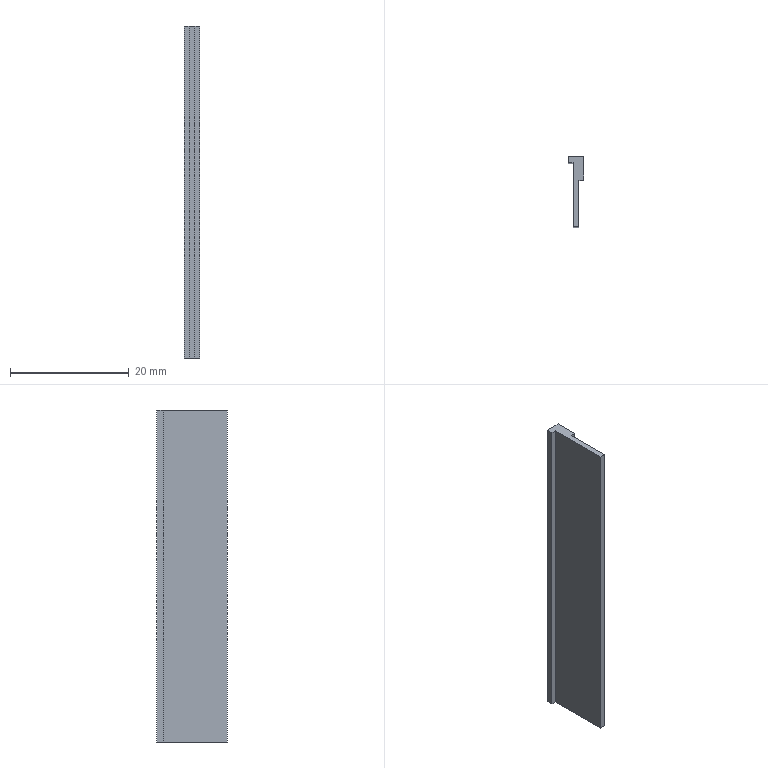Part | NX | features BREP 2 | 2 solids | 20 faces | box 2.58 x 11.896 x 56 mm | volume 1761 mm3 | plane 20
STEP:
#1=CARTESIAN_POINT('',(-0.4899,4.83,-4.));
#2=VERTEX_POINT('',#1);
#3=CARTESIAN_POINT('',(-0.4899,4.83,52.));
#4=VERTEX_POINT('',#3);
#5=CARTESIAN_POINT('',(-0.4899,4.83,0.));
#6=DIRECTION('',(0.,0.,1.));
#7=VECTOR('',#6,1000.);
#8=LINE('',#5,#7);
#9=EDGE_CURVE('',#2,#4,#8,.T.);
#10=ORIENTED_EDGE('',*,*,#9,.T.);
#11=CARTESIAN_POINT('',(-1.29,4.83,52.));
#12=VERTEX_POINT('',#11);
#13=CARTESIAN_POINT('',(-7.04,4.83,52.));
#14=DIRECTION('',(1.,0.,0.));
#15=VECTOR('',#14,1000.);
#16=LINE('',#13,#15);
#17=EDGE_CURVE('',#12,#4,#16,.T.);
#18=ORIENTED_EDGE('',*,*,#17,.F.);
#19=CARTESIAN_POINT('',(-1.29,4.83,-4.));
#20=VERTEX_POINT('',#19);
#21=CARTESIAN_POINT('',(-1.29,4.83,0.));
#22=DIRECTION('',(0.,0.,1.));
#23=VECTOR('',#22,1000.);
#24=LINE('',#21,#23);
#25=EDGE_CURVE('',#20,#12,#24,.T.);
#26=ORIENTED_EDGE('',*,*,#25,.F.);
#27=CARTESIAN_POINT('',(-7.04,4.83,-4.));
#28=DIRECTION('',(1.,0.,0.));
#29=VECTOR('',#28,1000.);
#30=LINE('',#27,#29);
#31=EDGE_CURVE('',#20,#2,#30,.T.);
#32=ORIENTED_EDGE('',*,*,#31,.T.);
#33=EDGE_LOOP('',(#10,#18,#26,#32));
#34=FACE_BOUND('',#33,.T.);
#35=CARTESIAN_POINT('',(-0.4899,4.83,0.));
#36=DIRECTION('',(0.,1.,0.));
#37=DIRECTION('',(1.,0.,0.));
#38=AXIS2_PLACEMENT_3D('',#35,#36,#37);
#39=PLANE('',#38);
#40=ADVANCED_FACE('',(#34),#39,.F.);
#41=ORIENTED_EDGE('',*,*,#25,.T.);
#42=CARTESIAN_POINT('',(-1.29,5.923,52.));
#43=VERTEX_POINT('',#42);
#44=CARTESIAN_POINT('',(-1.29,-19.679,52.));
#45=DIRECTION('',(0.,-1.,0.));
#46=VECTOR('',#45,1000.);
#47=LINE('',#44,#46);
#48=EDGE_CURVE('',#43,#12,#47,.T.);
#49=ORIENTED_EDGE('',*,*,#48,.F.);
#50=CARTESIAN_POINT('',(-1.29,5.923,-4.));
#51=VERTEX_POINT('',#50);
#52=CARTESIAN_POINT('',(-1.29,5.923,0.));
#53=DIRECTION('',(0.,0.,1.));
#54=VECTOR('',#53,1000.);
#55=LINE('',#52,#54);
#56=EDGE_CURVE('',#51,#43,#55,.T.);
#57=ORIENTED_EDGE('',*,*,#56,.F.);
#58=CARTESIAN_POINT('',(-1.29,-19.679,-4.));
#59=DIRECTION('',(0.,-1.,0.));
#60=VECTOR('',#59,1000.);
#61=LINE('',#58,#60);
#62=EDGE_CURVE('',#51,#20,#61,.T.);
#63=ORIENTED_EDGE('',*,*,#62,.T.);
#64=EDGE_LOOP('',(#41,#49,#57,#63));
#65=FACE_BOUND('',#64,.T.);
#66=CARTESIAN_POINT('',(-1.29,4.83,0.));
#67=DIRECTION('',(1.,0.,0.));
#68=DIRECTION('',(0.,-1.,0.));
#69=AXIS2_PLACEMENT_3D('',#66,#67,#68);
#70=PLANE('',#69);
#71=ADVANCED_FACE('',(#65),#70,.F.);
#72=ORIENTED_EDGE('',*,*,#56,.T.);
#73=CARTESIAN_POINT('',(1.29,5.923,52.));
#74=VERTEX_POINT('',#73);
#75=CARTESIAN_POINT('',(-7.04,5.923,52.));
#76=DIRECTION('',(-1.,0.,0.));
#77=VECTOR('',#76,1000.);
#78=LINE('',#75,#77);
#79=EDGE_CURVE('',#74,#43,#78,.T.);
#80=ORIENTED_EDGE('',*,*,#79,.F.);
#81=CARTESIAN_POINT('',(1.29,5.923,-4.));
#82=VERTEX_POINT('',#81);
#83=CARTESIAN_POINT('',(1.29,5.923,0.));
#84=DIRECTION('',(0.,0.,1.));
#85=VECTOR('',#84,1000.);
#86=LINE('',#83,#85);
#87=EDGE_CURVE('',#82,#74,#86,.T.);
#88=ORIENTED_EDGE('',*,*,#87,.F.);
#89=CARTESIAN_POINT('',(-7.04,5.923,-4.));
#90=DIRECTION('',(-1.,0.,0.));
#91=VECTOR('',#90,1000.);
#92=LINE('',#89,#91);
#93=EDGE_CURVE('',#82,#51,#92,.T.);
#94=ORIENTED_EDGE('',*,*,#93,.T.);
#95=EDGE_LOOP('',(#72,#80,#88,#94));
#96=FACE_BOUND('',#95,.T.);
#97=CARTESIAN_POINT('',(-7.04,5.923,0.));
#98=DIRECTION('',(0.,1.,0.));
#99=DIRECTION('',(1.,0.,0.));
#100=AXIS2_PLACEMENT_3D('',#97,#98,#99);
#101=PLANE('',#100);
#102=ADVANCED_FACE('',(#96),#101,.T.);
#103=ORIENTED_EDGE('',*,*,#87,.T.);
#104=CARTESIAN_POINT('',(1.29,1.93,52.));
#105=VERTEX_POINT('',#104);
#106=CARTESIAN_POINT('',(1.29,-19.679,52.));
#107=DIRECTION('',(0.,1.,0.));
#108=VECTOR('',#107,1000.);
#109=LINE('',#106,#108);
#110=EDGE_CURVE('',#105,#74,#109,.T.);
#111=ORIENTED_EDGE('',*,*,#110,.F.);
#112=CARTESIAN_POINT('',(1.29,1.93,-4.));
#113=VERTEX_POINT('',#112);
#114=CARTESIAN_POINT('',(1.29,1.93,0.));
#115=DIRECTION('',(0.,0.,1.));
#116=VECTOR('',#115,1000.);
#117=LINE('',#114,#116);
#118=EDGE_CURVE('',#113,#105,#117,.T.);
#119=ORIENTED_EDGE('',*,*,#118,.F.);
#120=CARTESIAN_POINT('',(1.29,-19.679,-4.));
#121=DIRECTION('',(0.,1.,0.));
#122=VECTOR('',#121,1000.);
#123=LINE('',#120,#122);
#124=EDGE_CURVE('',#113,#82,#123,.T.);
#125=ORIENTED_EDGE('',*,*,#124,.T.);
#126=EDGE_LOOP('',(#103,#111,#119,#125));
#127=FACE_BOUND('',#126,.T.);
#128=CARTESIAN_POINT('',(1.29,5.923,0.));
#129=DIRECTION('',(-1.,0.,0.));
#130=DIRECTION('',(0.,1.,0.));
#131=AXIS2_PLACEMENT_3D('',#128,#129,#130);
#132=PLANE('',#131);
#133=ADVANCED_FACE('',(#127),#132,.F.);
#134=ORIENTED_EDGE('',*,*,#118,.T.);
#135=CARTESIAN_POINT('',(0.4899,1.93,52.));
#136=VERTEX_POINT('',#135);
#137=CARTESIAN_POINT('',(-7.04,1.93,52.));
#138=DIRECTION('',(1.,0.,0.));
#139=VECTOR('',#138,1000.);
#140=LINE('',#137,#139);
#141=EDGE_CURVE('',#136,#105,#140,.T.);
#142=ORIENTED_EDGE('',*,*,#141,.F.);
#143=CARTESIAN_POINT('',(0.4899,1.93,-4.));
#144=VERTEX_POINT('',#143);
#145=CARTESIAN_POINT('',(0.4899,1.93,0.));
#146=DIRECTION('',(0.,0.,1.));
#147=VECTOR('',#146,1000.);
#148=LINE('',#145,#147);
#149=EDGE_CURVE('',#144,#136,#148,.T.);
#150=ORIENTED_EDGE('',*,*,#149,.F.);
#151=CARTESIAN_POINT('',(-7.04,1.93,-4.));
#152=DIRECTION('',(1.,0.,0.));
#153=VECTOR('',#152,1000.);
#154=LINE('',#151,#153);
#155=EDGE_CURVE('',#144,#113,#154,.T.);
#156=ORIENTED_EDGE('',*,*,#155,.T.);
#157=EDGE_LOOP('',(#134,#142,#150,#156));
#158=FACE_BOUND('',#157,.T.);
#159=CARTESIAN_POINT('',(1.29,1.93,0.));
#160=DIRECTION('',(0.,1.,0.));
#161=DIRECTION('',(1.,0.,0.));
#162=AXIS2_PLACEMENT_3D('',#159,#160,#161);
#163=PLANE('',#162);
#164=ADVANCED_FACE('',(#158),#163,.F.);
#165=CARTESIAN_POINT('',(0.4899,-5.973,-4.));
#166=VERTEX_POINT('',#165);
#167=CARTESIAN_POINT('',(0.4899,-5.973,52.));
#168=VERTEX_POINT('',#167);
#169=CARTESIAN_POINT('',(0.4899,-5.973,0.));
#170=DIRECTION('',(0.,0.,1.));
#171=VECTOR('',#170,1000.);
#172=LINE('',#169,#171);
#173=EDGE_CURVE('',#166,#168,#172,.T.);
#174=ORIENTED_EDGE('',*,*,#173,.F.);
#175=CARTESIAN_POINT('',(0.4899,-19.679,-4.));
#176=DIRECTION('',(0.,1.,0.));
#177=VECTOR('',#176,1000.);
#178=LINE('',#175,#177);
#179=EDGE_CURVE('',#166,#144,#178,.T.);
#180=ORIENTED_EDGE('',*,*,#179,.T.);
#181=ORIENTED_EDGE('',*,*,#149,.T.);
#182=CARTESIAN_POINT('',(0.4899,-19.679,52.));
#183=DIRECTION('',(0.,1.,0.));
#184=VECTOR('',#183,1000.);
#185=LINE('',#182,#184);
#186=EDGE_CURVE('',#168,#136,#185,.T.);
#187=ORIENTED_EDGE('',*,*,#186,.F.);
#188=EDGE_LOOP('',(#174,#180,#181,#187));
#189=FACE_BOUND('',#188,.T.);
#190=CARTESIAN_POINT('',(0.4899,-5.28,0.));
#191=DIRECTION('',(-1.,0.,0.));
#192=DIRECTION('',(0.,1.,0.));
#193=AXIS2_PLACEMENT_3D('',#190,#191,#192);
#194=PLANE('',#193);
#195=ADVANCED_FACE('',(#189),#194,.F.);
#196=ORIENTED_EDGE('',*,*,#173,.T.);
#197=CARTESIAN_POINT('',(-0.4899,-5.973,52.));
#198=VERTEX_POINT('',#197);
#199=CARTESIAN_POINT('',(-7.04,-5.973,52.));
#200=DIRECTION('',(1.,0.,0.));
#201=VECTOR('',#200,1000.);
#202=LINE('',#199,#201);
#203=EDGE_CURVE('',#198,#168,#202,.T.);
#204=ORIENTED_EDGE('',*,*,#203,.F.);
#205=CARTESIAN_POINT('',(-0.4899,-5.973,-4.));
#206=VERTEX_POINT('',#205);
#207=CARTESIAN_POINT('',(-0.4899,-5.973,0.));
#208=DIRECTION('',(0.,0.,1.));
#209=VECTOR('',#208,1000.);
#210=LINE('',#207,#209);
#211=EDGE_CURVE('',#206,#198,#210,.T.);
#212=ORIENTED_EDGE('',*,*,#211,.F.);
#213=CARTESIAN_POINT('',(-7.04,-5.973,-4.));
#214=DIRECTION('',(1.,0.,0.));
#215=VECTOR('',#214,1000.);
#216=LINE('',#213,#215);
#217=EDGE_CURVE('',#206,#166,#216,.T.);
#218=ORIENTED_EDGE('',*,*,#217,.T.);
#219=EDGE_LOOP('',(#196,#204,#212,#218));
#220=FACE_BOUND('',#219,.T.);
#221=CARTESIAN_POINT('',(-7.04,-5.973,0.));
#222=DIRECTION('',(0.,-1.,0.));
#223=DIRECTION('',(-1.,0.,0.));
#224=AXIS2_PLACEMENT_3D('',#221,#222,#223);
#225=PLANE('',#224);
#226=ADVANCED_FACE('',(#220),#225,.T.);
#227=CARTESIAN_POINT('',(-0.4899,-19.679,-4.));
#228=DIRECTION('',(0.,-1.,0.));
#229=VECTOR('',#228,1000.);
#230=LINE('',#227,#229);
#231=EDGE_CURVE('',#2,#206,#230,.T.);
#232=ORIENTED_EDGE('',*,*,#231,.T.);
#233=ORIENTED_EDGE('',*,*,#211,.T.);
#234=CARTESIAN_POINT('',(-0.4899,-19.679,52.));
#235=DIRECTION('',(0.,-1.,0.));
#236=VECTOR('',#235,1000.);
#237=LINE('',#234,#236);
#238=EDGE_CURVE('',#4,#198,#237,.T.);
#239=ORIENTED_EDGE('',*,*,#238,.F.);
#240=ORIENTED_EDGE('',*,*,#9,.F.);
#241=EDGE_LOOP('',(#232,#233,#239,#240));
#242=FACE_BOUND('',#241,.T.);
#243=CARTESIAN_POINT('',(-0.4899,-2.38,0.));
#244=DIRECTION('',(1.,0.,0.));
#245=DIRECTION('',(0.,-1.,0.));
#246=AXIS2_PLACEMENT_3D('',#243,#244,#245);
#247=PLANE('',#246);
#248=ADVANCED_FACE('',(#242),#247,.F.);
#249=ORIENTED_EDGE('',*,*,#238,.T.);
#250=ORIENTED_EDGE('',*,*,#203,.T.);
#251=ORIENTED_EDGE('',*,*,#186,.T.);
#252=ORIENTED_EDGE('',*,*,#141,.T.);
#253=ORIENTED_EDGE('',*,*,#110,.T.);
#254=ORIENTED_EDGE('',*,*,#79,.T.);
#255=ORIENTED_EDGE('',*,*,#48,.T.);
#256=ORIENTED_EDGE('',*,*,#17,.T.);
#257=EDGE_LOOP('',(#249,#250,#251,#252,#253,#254,#255,#256));
#258=FACE_BOUND('',#257,.T.);
#259=CARTESIAN_POINT('',(-7.04,-19.679,52.));
#260=DIRECTION('',(0.,0.,1.));
#261=DIRECTION('',(-1.,0.,0.));
#262=AXIS2_PLACEMENT_3D('',#259,#260,#261);
#263=PLANE('',#262);
#264=ADVANCED_FACE('',(#258),#263,.T.);
#265=ORIENTED_EDGE('',*,*,#217,.F.);
#266=ORIENTED_EDGE('',*,*,#231,.F.);
#267=ORIENTED_EDGE('',*,*,#31,.F.);
#268=ORIENTED_EDGE('',*,*,#62,.F.);
#269=ORIENTED_EDGE('',*,*,#93,.F.);
#270=ORIENTED_EDGE('',*,*,#124,.F.);
#271=ORIENTED_EDGE('',*,*,#155,.F.);
#272=ORIENTED_EDGE('',*,*,#179,.F.);
#273=EDGE_LOOP('',(#265,#266,#267,#268,#269,#270,#271,#272));
#274=FACE_BOUND('',#273,.T.);
#275=CARTESIAN_POINT('',(-7.04,-19.679,-4.));
#276=DIRECTION('',(0.,0.,1.));
#277=DIRECTION('',(-1.,0.,0.));
#278=AXIS2_PLACEMENT_3D('',#275,#276,#277);
#279=PLANE('',#278);
#280=ADVANCED_FACE('',(#274),#279,.F.);
#281=CLOSED_SHELL('',(#40,#71,#102,#133,#164,#195,#226,#248,#264,#280));
#282=MANIFOLD_SOLID_BREP('',#281);
#283=CARTESIAN_POINT('',(-0.4899,4.83,-4.));
#284=VERTEX_POINT('',#283);
#285=CARTESIAN_POINT('',(-0.4899,4.83,52.));
#286=VERTEX_POINT('',#285);
#287=CARTESIAN_POINT('',(-0.4899,4.83,0.));
#288=DIRECTION('',(0.,0.,1.));
#289=VECTOR('',#288,1000.);
#290=LINE('',#287,#289);
#291=EDGE_CURVE('',#284,#286,#290,.T.);
#292=ORIENTED_EDGE('',*,*,#291,.T.);
#293=CARTESIAN_POINT('',(-1.29,4.83,52.));
#294=VERTEX_POINT('',#293);
#295=CARTESIAN_POINT('',(-7.04,4.83,52.));
#296=DIRECTION('',(1.,0.,0.));
#297=VECTOR('',#296,1000.);
#298=LINE('',#295,#297);
#299=EDGE_CURVE('',#294,#286,#298,.T.);
#300=ORIENTED_EDGE('',*,*,#299,.F.);
#301=CARTESIAN_POINT('',(-1.29,4.83,-4.));
#302=VERTEX_POINT('',#301);
#303=CARTESIAN_POINT('',(-1.29,4.83,0.));
#304=DIRECTION('',(0.,0.,1.));
#305=VECTOR('',#304,1000.);
#306=LINE('',#303,#305);
#307=EDGE_CURVE('',#302,#294,#306,.T.);
#308=ORIENTED_EDGE('',*,*,#307,.F.);
#309=CARTESIAN_POINT('',(-7.04,4.83,-4.));
#310=DIRECTION('',(1.,0.,0.));
#311=VECTOR('',#310,1000.);
#312=LINE('',#309,#311);
#313=EDGE_CURVE('',#302,#284,#312,.T.);
#314=ORIENTED_EDGE('',*,*,#313,.T.);
#315=EDGE_LOOP('',(#292,#300,#308,#314));
#316=FACE_BOUND('',#315,.T.);
#317=CARTESIAN_POINT('',(-0.4899,4.83,0.));
#318=DIRECTION('',(0.,1.,0.));
#319=DIRECTION('',(1.,0.,0.));
#320=AXIS2_PLACEMENT_3D('',#317,#318,#319);
#321=PLANE('',#320);
#322=ADVANCED_FACE('',(#316),#321,.F.);
#323=ORIENTED_EDGE('',*,*,#307,.T.);
#324=CARTESIAN_POINT('',(-1.29,5.923,52.));
#325=VERTEX_POINT('',#324);
#326=CARTESIAN_POINT('',(-1.29,-19.679,52.));
#327=DIRECTION('',(0.,-1.,0.));
#328=VECTOR('',#327,1000.);
#329=LINE('',#326,#328);
#330=EDGE_CURVE('',#325,#294,#329,.T.);
#331=ORIENTED_EDGE('',*,*,#330,.F.);
#332=CARTESIAN_POINT('',(-1.29,5.923,-4.));
#333=VERTEX_POINT('',#332);
#334=CARTESIAN_POINT('',(-1.29,5.923,0.));
#335=DIRECTION('',(0.,0.,1.));
#336=VECTOR('',#335,1000.);
#337=LINE('',#334,#336);
#338=EDGE_CURVE('',#333,#325,#337,.T.);
#339=ORIENTED_EDGE('',*,*,#338,.F.);
#340=CARTESIAN_POINT('',(-1.29,-19.679,-4.));
#341=DIRECTION('',(0.,-1.,0.));
#342=VECTOR('',#341,1000.);
#343=LINE('',#340,#342);
#344=EDGE_CURVE('',#333,#302,#343,.T.);
#345=ORIENTED_EDGE('',*,*,#344,.T.);
#346=EDGE_LOOP('',(#323,#331,#339,#345));
#347=FACE_BOUND('',#346,.T.);
#348=CARTESIAN_POINT('',(-1.29,4.83,0.));
#349=DIRECTION('',(1.,0.,0.));
#350=DIRECTION('',(0.,-1.,0.));
#351=AXIS2_PLACEMENT_3D('',#348,#349,#350);
#352=PLANE('',#351);
#353=ADVANCED_FACE('',(#347),#352,.F.);
#354=ORIENTED_EDGE('',*,*,#338,.T.);
#355=CARTESIAN_POINT('',(1.29,5.923,52.));
#356=VERTEX_POINT('',#355);
#357=CARTESIAN_POINT('',(-7.04,5.923,52.));
#358=DIRECTION('',(-1.,0.,0.));
#359=VECTOR('',#358,1000.);
#360=LINE('',#357,#359);
#361=EDGE_CURVE('',#356,#325,#360,.T.);
#362=ORIENTED_EDGE('',*,*,#361,.F.);
#363=CARTESIAN_POINT('',(1.29,5.923,-4.));
#364=VERTEX_POINT('',#363);
#365=CARTESIAN_POINT('',(1.29,5.923,0.));
#366=DIRECTION('',(0.,0.,1.));
#367=VECTOR('',#366,1000.);
#368=LINE('',#365,#367);
#369=EDGE_CURVE('',#364,#356,#368,.T.);
#370=ORIENTED_EDGE('',*,*,#369,.F.);
#371=CARTESIAN_POINT('',(-7.04,5.923,-4.));
#372=DIRECTION('',(-1.,0.,0.));
#373=VECTOR('',#372,1000.);
#374=LINE('',#371,#373);
#375=EDGE_CURVE('',#364,#333,#374,.T.);
#376=ORIENTED_EDGE('',*,*,#375,.T.);
#377=EDGE_LOOP('',(#354,#362,#370,#376));
#378=FACE_BOUND('',#377,.T.);
#379=CARTESIAN_POINT('',(-7.04,5.923,0.));
#380=DIRECTION('',(0.,1.,0.));
#381=DIRECTION('',(1.,0.,0.));
#382=AXIS2_PLACEMENT_3D('',#379,#380,#381);
#383=PLANE('',#382);
#384=ADVANCED_FACE('',(#378),#383,.T.);
#385=ORIENTED_EDGE('',*,*,#369,.T.);
#386=CARTESIAN_POINT('',(1.29,1.93,52.));
#387=VERTEX_POINT('',#386);
#388=CARTESIAN_POINT('',(1.29,-19.679,52.));
#389=DIRECTION('',(0.,1.,0.));
#390=VECTOR('',#389,1000.);
#391=LINE('',#388,#390);
#392=EDGE_CURVE('',#387,#356,#391,.T.);
#393=ORIENTED_EDGE('',*,*,#392,.F.);
#394=CARTESIAN_POINT('',(1.29,1.93,-4.));
#395=VERTEX_POINT('',#394);
#396=CARTESIAN_POINT('',(1.29,1.93,0.));
#397=DIRECTION('',(0.,0.,1.));
#398=VECTOR('',#397,1000.);
#399=LINE('',#396,#398);
#400=EDGE_CURVE('',#395,#387,#399,.T.);
#401=ORIENTED_EDGE('',*,*,#400,.F.);
#402=CARTESIAN_POINT('',(1.29,-19.679,-4.));
#403=DIRECTION('',(0.,1.,0.));
#404=VECTOR('',#403,1000.);
#405=LINE('',#402,#404);
#406=EDGE_CURVE('',#395,#364,#405,.T.);
#407=ORIENTED_EDGE('',*,*,#406,.T.);
#408=EDGE_LOOP('',(#385,#393,#401,#407));
#409=FACE_BOUND('',#408,.T.);
#410=CARTESIAN_POINT('',(1.29,5.923,0.));
#411=DIRECTION('',(-1.,0.,0.));
#412=DIRECTION('',(0.,1.,0.));
#413=AXIS2_PLACEMENT_3D('',#410,#411,#412);
#414=PLANE('',#413);
#415=ADVANCED_FACE('',(#409),#414,.F.);
#416=ORIENTED_EDGE('',*,*,#400,.T.);
#417=CARTESIAN_POINT('',(0.4899,1.93,52.));
#418=VERTEX_POINT('',#417);
#419=CARTESIAN_POINT('',(-7.04,1.93,52.));
#420=DIRECTION('',(1.,0.,0.));
#421=VECTOR('',#420,1000.);
#422=LINE('',#419,#421);
#423=EDGE_CURVE('',#418,#387,#422,.T.);
#424=ORIENTED_EDGE('',*,*,#423,.F.);
#425=CARTESIAN_POINT('',(0.4899,1.93,-4.));
#426=VERTEX_POINT('',#425);
#427=CARTESIAN_POINT('',(0.4899,1.93,0.));
#428=DIRECTION('',(0.,0.,1.));
#429=VECTOR('',#428,1000.);
#430=LINE('',#427,#429);
#431=EDGE_CURVE('',#426,#418,#430,.T.);
#432=ORIENTED_EDGE('',*,*,#431,.F.);
#433=CARTESIAN_POINT('',(-7.04,1.93,-4.));
#434=DIRECTION('',(1.,0.,0.));
#435=VECTOR('',#434,1000.);
#436=LINE('',#433,#435);
#437=EDGE_CURVE('',#426,#395,#436,.T.);
#438=ORIENTED_EDGE('',*,*,#437,.T.);
#439=EDGE_LOOP('',(#416,#424,#432,#438));
#440=FACE_BOUND('',#439,.T.);
#441=CARTESIAN_POINT('',(1.29,1.93,0.));
#442=DIRECTION('',(0.,1.,0.));
#443=DIRECTION('',(1.,0.,0.));
#444=AXIS2_PLACEMENT_3D('',#441,#442,#443);
#445=PLANE('',#444);
#446=ADVANCED_FACE('',(#440),#445,.F.);
#447=CARTESIAN_POINT('',(0.4899,-5.973,-4.));
#448=VERTEX_POINT('',#447);
#449=CARTESIAN_POINT('',(0.4899,-5.973,52.));
#450=VERTEX_POINT('',#449);
#451=CARTESIAN_POINT('',(0.4899,-5.973,0.));
#452=DIRECTION('',(0.,0.,1.));
#453=VECTOR('',#452,1000.);
#454=LINE('',#451,#453);
#455=EDGE_CURVE('',#448,#450,#454,.T.);
#456=ORIENTED_EDGE('',*,*,#455,.F.);
#457=CARTESIAN_POINT('',(0.4899,-19.679,-4.));
#458=DIRECTION('',(0.,1.,0.));
#459=VECTOR('',#458,1000.);
#460=LINE('',#457,#459);
#461=EDGE_CURVE('',#448,#426,#460,.T.);
#462=ORIENTED_EDGE('',*,*,#461,.T.);
#463=ORIENTED_EDGE('',*,*,#431,.T.);
#464=CARTESIAN_POINT('',(0.4899,-19.679,52.));
#465=DIRECTION('',(0.,1.,0.));
#466=VECTOR('',#465,1000.);
#467=LINE('',#464,#466);
#468=EDGE_CURVE('',#450,#418,#467,.T.);
#469=ORIENTED_EDGE('',*,*,#468,.F.);
#470=EDGE_LOOP('',(#456,#462,#463,#469));
#471=FACE_BOUND('',#470,.T.);
#472=CARTESIAN_POINT('',(0.4899,-5.28,0.));
#473=DIRECTION('',(-1.,0.,0.));
#474=DIRECTION('',(0.,1.,0.));
#475=AXIS2_PLACEMENT_3D('',#472,#473,#474);
#476=PLANE('',#475);
#477=ADVANCED_FACE('',(#471),#476,.F.);
#478=ORIENTED_EDGE('',*,*,#455,.T.);
#479=CARTESIAN_POINT('',(-0.4899,-5.973,52.));
#480=VERTEX_POINT('',#479);
#481=CARTESIAN_POINT('',(-7.04,-5.973,52.));
#482=DIRECTION('',(1.,0.,0.));
#483=VECTOR('',#482,1000.);
#484=LINE('',#481,#483);
#485=EDGE_CURVE('',#480,#450,#484,.T.);
#486=ORIENTED_EDGE('',*,*,#485,.F.);
#487=CARTESIAN_POINT('',(-0.4899,-5.973,-4.));
#488=VERTEX_POINT('',#487);
#489=CARTESIAN_POINT('',(-0.4899,-5.973,0.));
#490=DIRECTION('',(0.,0.,1.));
#491=VECTOR('',#490,1000.);
#492=LINE('',#489,#491);
#493=EDGE_CURVE('',#488,#480,#492,.T.);
#494=ORIENTED_EDGE('',*,*,#493,.F.);
#495=CARTESIAN_POINT('',(-7.04,-5.973,-4.));
#496=DIRECTION('',(1.,0.,0.));
#497=VECTOR('',#496,1000.);
#498=LINE('',#495,#497);
#499=EDGE_CURVE('',#488,#448,#498,.T.);
#500=ORIENTED_EDGE('',*,*,#499,.T.);
#501=EDGE_LOOP('',(#478,#486,#494,#500));
#502=FACE_BOUND('',#501,.T.);
#503=CARTESIAN_POINT('',(-7.04,-5.973,0.));
#504=DIRECTION('',(0.,-1.,0.));
#505=DIRECTION('',(-1.,0.,0.));
#506=AXIS2_PLACEMENT_3D('',#503,#504,#505);
#507=PLANE('',#506);
#508=ADVANCED_FACE('',(#502),#507,.T.);
#509=CARTESIAN_POINT('',(-0.4899,-19.679,-4.));
#510=DIRECTION('',(0.,-1.,0.));
#511=VECTOR('',#510,1000.);
#512=LINE('',#509,#511);
#513=EDGE_CURVE('',#284,#488,#512,.T.);
#514=ORIENTED_EDGE('',*,*,#513,.T.);
#515=ORIENTED_EDGE('',*,*,#493,.T.);
#516=CARTESIAN_POINT('',(-0.4899,-19.679,52.));
#517=DIRECTION('',(0.,-1.,0.));
#518=VECTOR('',#517,1000.);
#519=LINE('',#516,#518);
#520=EDGE_CURVE('',#286,#480,#519,.T.);
#521=ORIENTED_EDGE('',*,*,#520,.F.);
#522=ORIENTED_EDGE('',*,*,#291,.F.);
#523=EDGE_LOOP('',(#514,#515,#521,#522));
#524=FACE_BOUND('',#523,.T.);
#525=CARTESIAN_POINT('',(-0.4899,-2.38,0.));
#526=DIRECTION('',(1.,0.,0.));
#527=DIRECTION('',(0.,-1.,0.));
#528=AXIS2_PLACEMENT_3D('',#525,#526,#527);
#529=PLANE('',#528);
#530=ADVANCED_FACE('',(#524),#529,.F.);
#531=ORIENTED_EDGE('',*,*,#520,.T.);
#532=ORIENTED_EDGE('',*,*,#485,.T.);
#533=ORIENTED_EDGE('',*,*,#468,.T.);
#534=ORIENTED_EDGE('',*,*,#423,.T.);
#535=ORIENTED_EDGE('',*,*,#392,.T.);
#536=ORIENTED_EDGE('',*,*,#361,.T.);
#537=ORIENTED_EDGE('',*,*,#330,.T.);
#538=ORIENTED_EDGE('',*,*,#299,.T.);
#539=EDGE_LOOP('',(#531,#532,#533,#534,#535,#536,#537,#538));
#540=FACE_BOUND('',#539,.T.);
#541=CARTESIAN_POINT('',(-7.04,-19.679,52.));
#542=DIRECTION('',(0.,0.,1.));
#543=DIRECTION('',(-1.,0.,0.));
#544=AXIS2_PLACEMENT_3D('',#541,#542,#543);
#545=PLANE('',#544);
#546=ADVANCED_FACE('',(#540),#545,.T.);
#547=ORIENTED_EDGE('',*,*,#499,.F.);
#548=ORIENTED_EDGE('',*,*,#513,.F.);
#549=ORIENTED_EDGE('',*,*,#313,.F.);
#550=ORIENTED_EDGE('',*,*,#344,.F.);
#551=ORIENTED_EDGE('',*,*,#375,.F.);
#552=ORIENTED_EDGE('',*,*,#406,.F.);
#553=ORIENTED_EDGE('',*,*,#437,.F.);
#554=ORIENTED_EDGE('',*,*,#461,.F.);
#555=EDGE_LOOP('',(#547,#548,#549,#550,#551,#552,#553,#554));
#556=FACE_BOUND('',#555,.T.);
#557=CARTESIAN_POINT('',(-7.04,-19.679,-4.));
#558=DIRECTION('',(0.,0.,1.));
#559=DIRECTION('',(-1.,0.,0.));
#560=AXIS2_PLACEMENT_3D('',#557,#558,#559);
#561=PLANE('',#560);
#562=ADVANCED_FACE('',(#556),#561,.F.);
#563=CLOSED_SHELL('',(#322,#353,#384,#415,#446,#477,#508,#530,#546,#562));
#564=MANIFOLD_SOLID_BREP('',#563);
#565=(LENGTH_UNIT()NAMED_UNIT(*)SI_UNIT(.MILLI.,.METRE.));
#566=UNCERTAINTY_MEASURE_WITH_UNIT(LENGTH_MEASURE(0.00001),#565,'','');
#567=(NAMED_UNIT(*)PLANE_ANGLE_UNIT()SI_UNIT($,.RADIAN.));
#568=(NAMED_UNIT(*)SI_UNIT($,.STERADIAN.)SOLID_ANGLE_UNIT());
#569=(GEOMETRIC_REPRESENTATION_CONTEXT(3)GLOBAL_UNCERTAINTY_ASSIGNED_CONTEXT((#566))GLOBAL_UNIT_ASSIGNED_CONTEXT((#565,#567,#568))REPRESENTATION_CONTEXT('',''));
#570=ADVANCED_BREP_SHAPE_REPRESENTATION('',(#282,#564),#569);